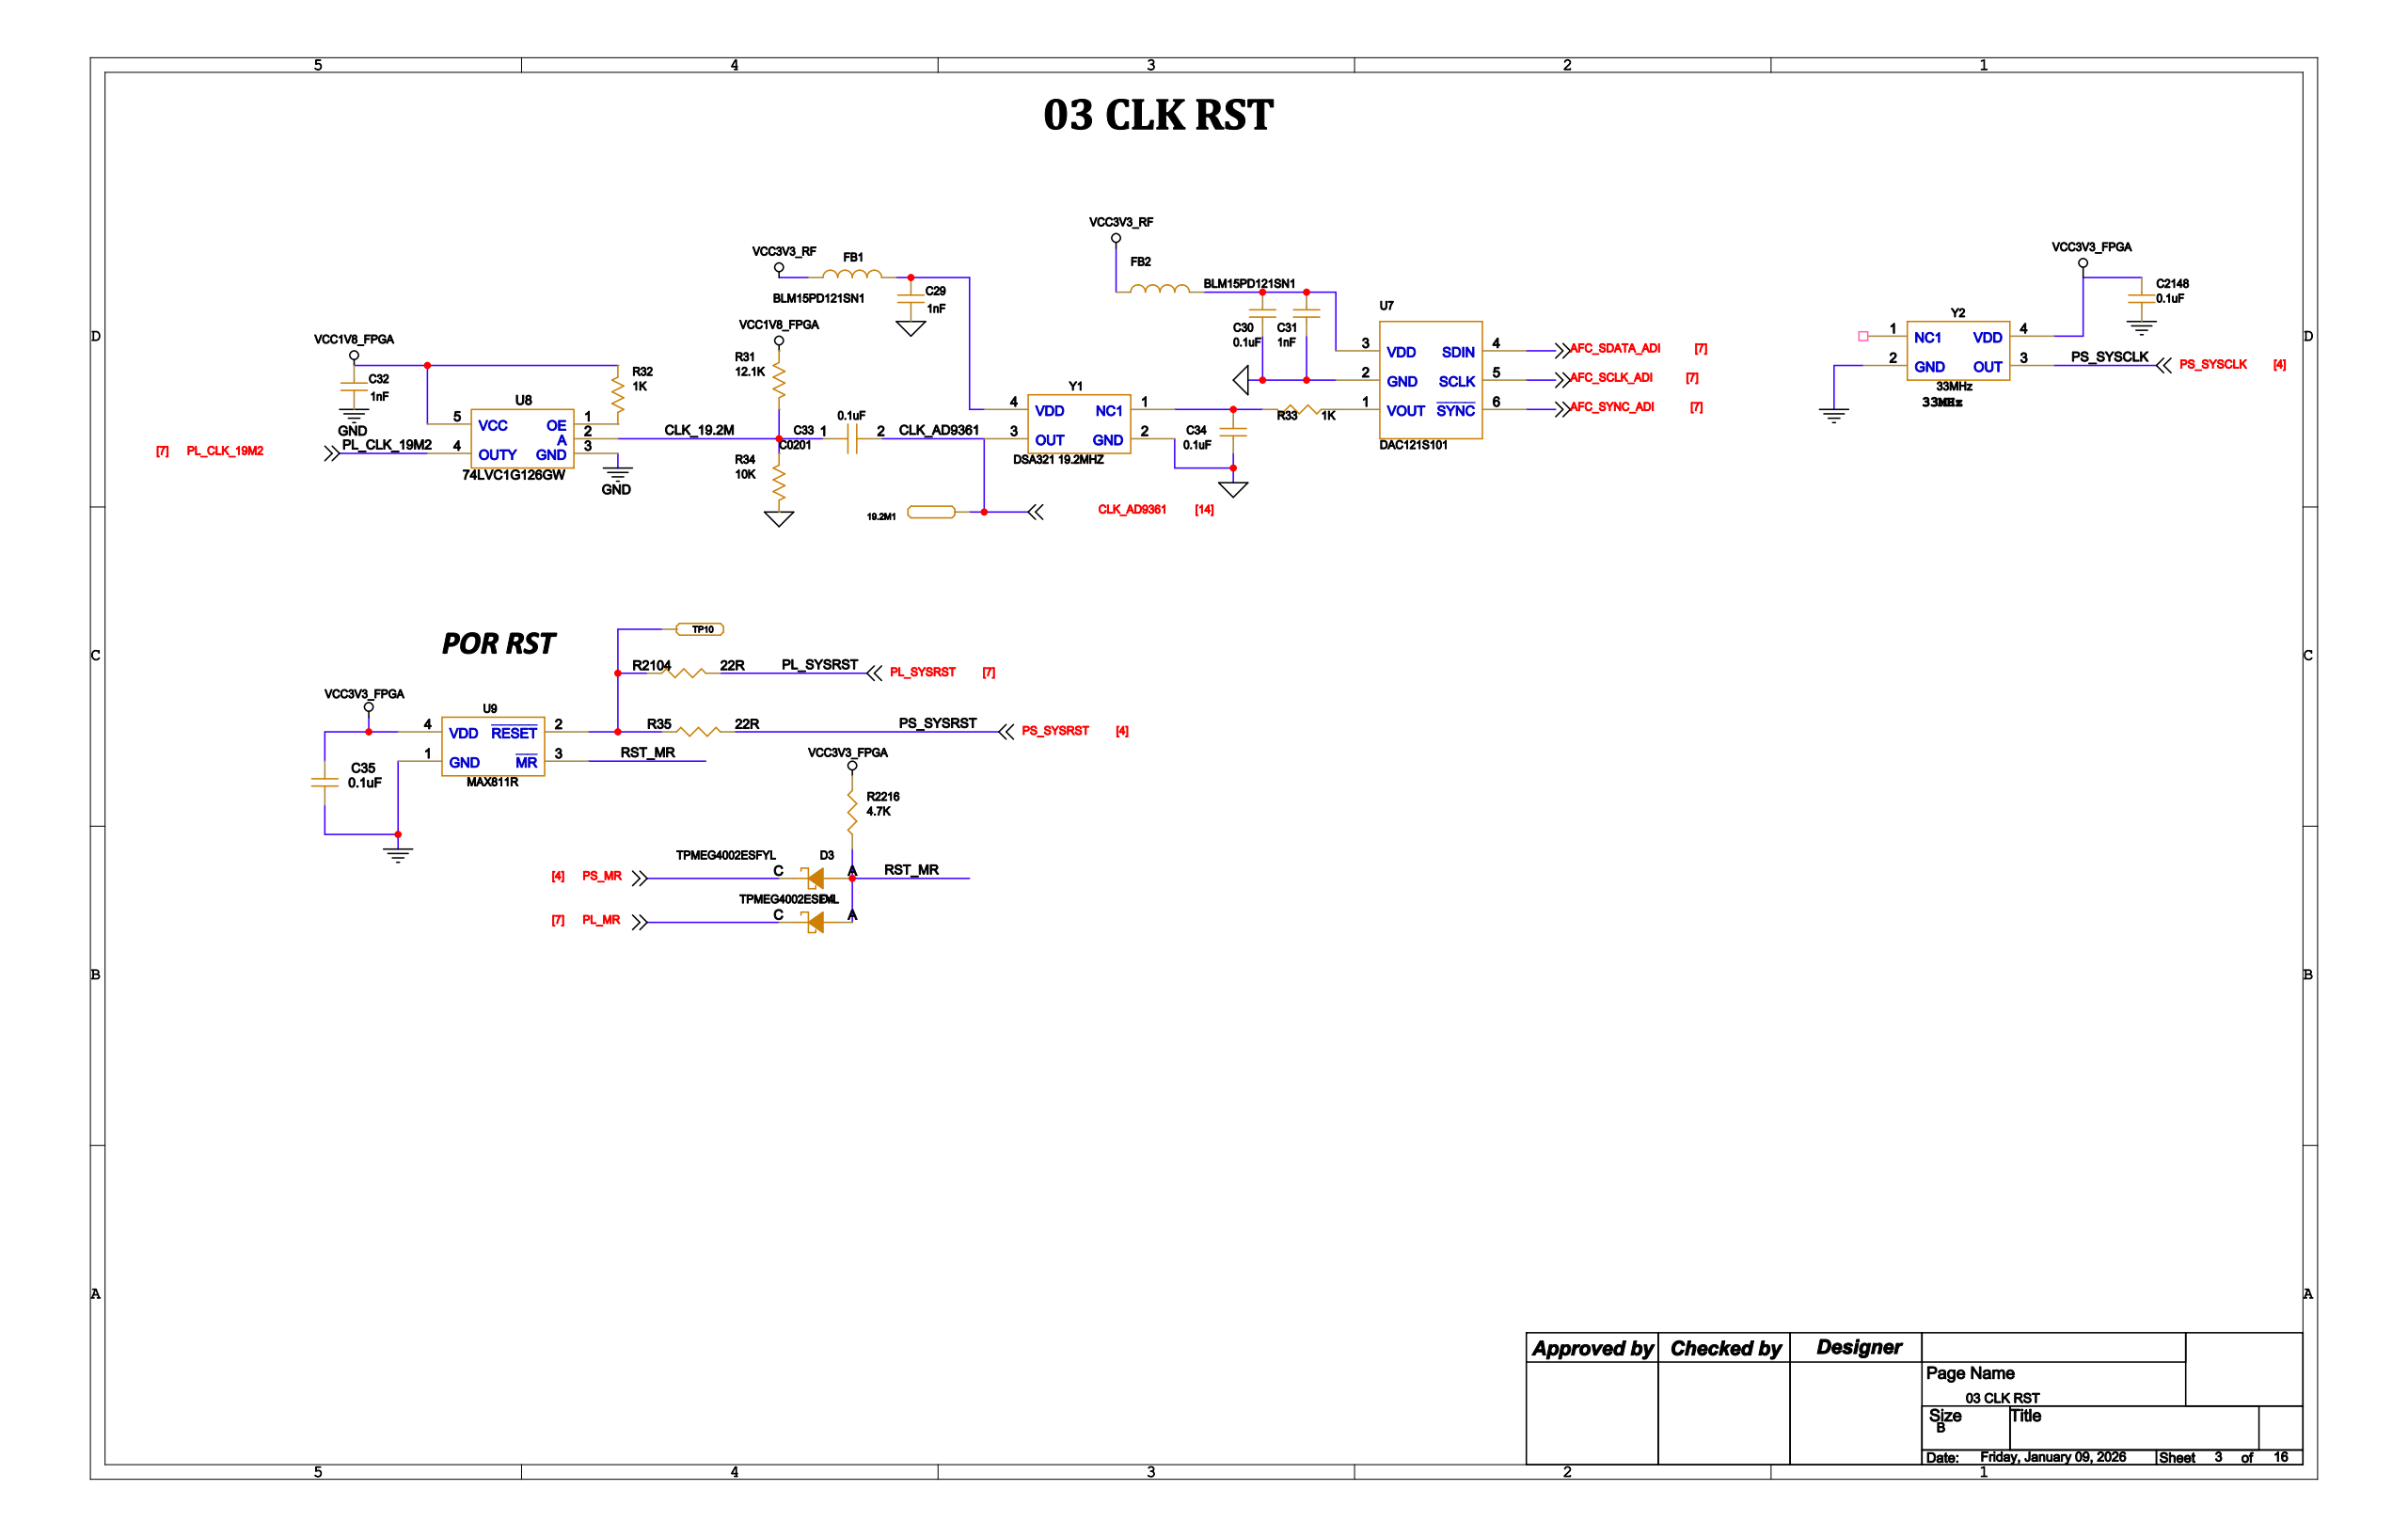Circuit board | Cadence Allegro | 442 parts | 326 nets | one sheet of the schematic
Parts on this sheet (reference | value | footprint):
19.2M1 | LABTESTPOINT | LTPT28C49P
C29 | 1nF | C0201
C30 | 0.1uF | C0201
C31 | 1nF | C0201
C32 | 1nF | C0201
C33 | 0.1uF | C0201
C34 | 0.1uF | C0201
C35 | 0.1uF | C0201
C2148 | 0.1uF | C0201
D3 | TPMEG4002ESFYL | D0201
D4 | TPMEG4002ESFYL | D0201
FB1 | BLM15PD121SN1 | L0402_D
FB2 | BLM15PD121SN1 | L0402_D
R31 | 12.1K | R0201
R32 | 1K | R0201
R33 | 1K | R0201
R34 | 10K | R0201
R35 | 22R | R0201
R2104 | 22R | R0201
R2216 | 4.7K | R0201
TP10 | LABTESTPOINT | LTPT28C49P
U7 | DAC121S101 | SOT-23-6
U8 | 74LVC1G126GW | SC-70
U9 | MAX811R | SOT-143
Y1 | DSA321 19.2MHZ | OSC2520
Y2 | 33MHz | OSC2520
Nets of these parts (net: part-pin ...):
GND: C29-2 C30-2 C31-2 C32-2 C34-1 C35-2 C2148-2 R34-2 U7-2 U8-3 U9-1 Y1-2 Y2-2
VCC3V3_RF: FB1-2 FB2-2
VCC1V8_FPGA: C32-1 R31-1 R32-2 U8-5
RST_MR: D3-A D4-A R2216-2 U9-3
PS_MR: D3-C
PL_MR: D4-C
VCC3V3_FPGA: C35-1 C2148-1 R2216-1 U9-4 Y2-4
N16754546: C34-2 R33-2 Y1-1
CLK_AD9361: 19.2M1-1 C33-2 Y1-3
N16754836: C29-1 FB1-1 Y1-4
PS_SYSCLK: Y2-3
N16754566: C30-1 C31-1 FB2-1 U7-3
CLK_19.2M: C33-1 R31-2 R34-1 U8-2
PL_SYSRST: R2104-1
N48900066: R35-2 R2104-2 TP10-1 U9-2
PS_SYSRST: R35-1
N490074890: R32-1 U8-1
N416338810: R33-1 U7-1
PL_CLK_19M2: U8-4
AFC_SCLK_ADI: U7-5
AFC_SDATA_ADI: U7-4
AFC_SYNC_ADI: U7-6